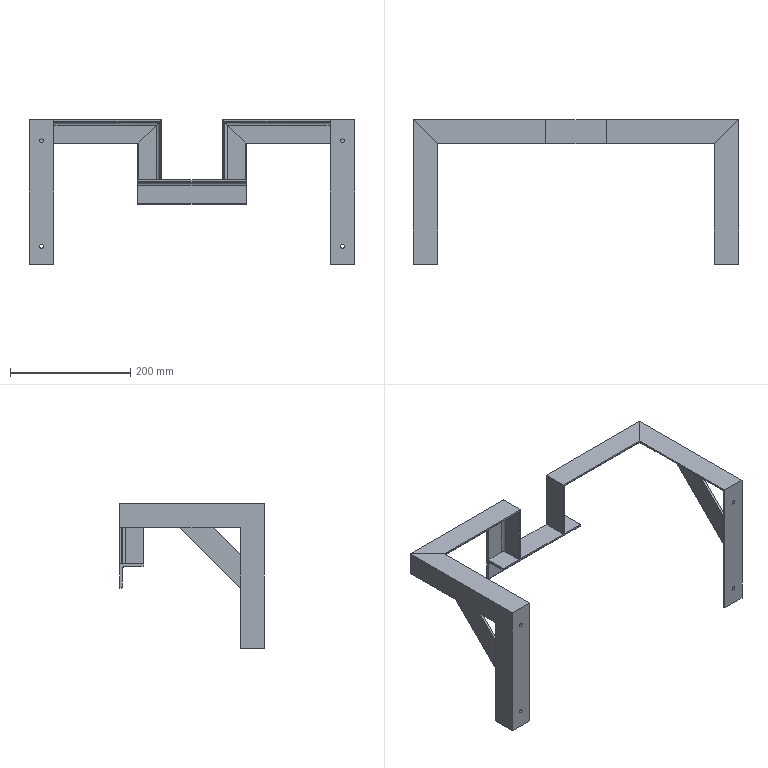Part | SolidWorks | features ICE 2, 3DProfileFeature 1, MirrorPattern 1, WeldMemberFeat 1, WeldmentFeature 1 | 9 solids | 115 faces | box 540 x 240 x 240 mm | volume 569268 mm3 | plane 80 | cylinder 35 | commonest cylinder face diameters 2.667 x18 10 x9 6.5 x8